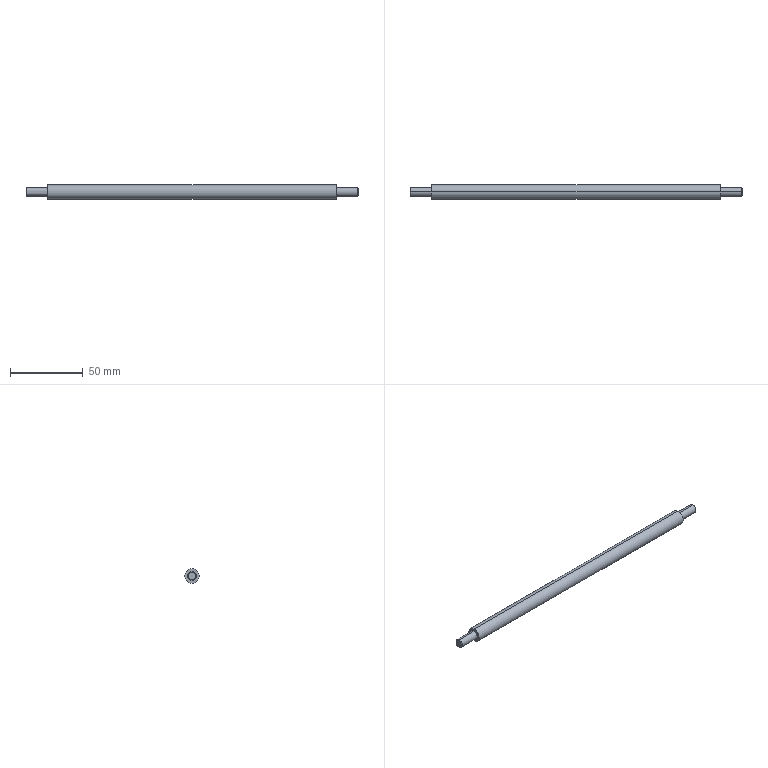Part | STEP file | sliding shaft_SUS304 | 1 solid | 14 faces | box 228 x 10 x 10 mm | volume 16395 mm3 | cylinder 6 | cone 4 | plane 4 | commonest cylinder face diameters 6 x4 10 x2
STEP:
#1=CARTESIAN_POINT('',(0.,0.,0.));
#2=DIRECTION('',(0.,0.,1.));
#3=DIRECTION('',(1.,0.,0.));
#4=AXIS2_PLACEMENT_3D('',#1,#2,#3);
#5=CARTESIAN_POINT('',(198.,0.,5.));
#6=VERTEX_POINT('',#5);
#7=CARTESIAN_POINT('',(198.,0.,-5.));
#8=VERTEX_POINT('',#7);
#9=CARTESIAN_POINT('',(198.,0.,0.));
#10=DIRECTION('',(-1.,0.,0.));
#11=DIRECTION('',(0.,0.,1.));
#12=AXIS2_PLACEMENT_3D('',#9,#10,#11);
#13=CIRCLE('',#12,5.);
#14=CARTESIAN_POINT('',(198.,0.,0.));
#15=DIRECTION('',(-1.,0.,0.));
#16=DIRECTION('',(0.,0.,1.));
#17=AXIS2_PLACEMENT_3D('',#14,#15,#16);
#18=CYLINDRICAL_SURFACE('',#17,5.);
#19=CARTESIAN_POINT('',(0.,0.));
#20=DIRECTION('',(1.,0.));
#21=VECTOR('',#20,1.);
#22=LINE('',#19,#21);
#23=(GEOMETRIC_REPRESENTATION_CONTEXT(2)PARAMETRIC_REPRESENTATION_CONTEXT()REPRESENTATION_CONTEXT('',''));
#24=DEFINITIONAL_REPRESENTATION('',(#22),#23);
#25=PCURVE('',#18,#24);
#26=CARTESIAN_POINT('',(198.,0.,0.));
#27=DIRECTION('',(1.,0.,0.));
#28=DIRECTION('',(0.,0.,-1.));
#29=AXIS2_PLACEMENT_3D('',#26,#27,#28);
#30=PLANE('',#29);
#31=CARTESIAN_POINT('',(-5.,0.));
#32=CARTESIAN_POINT('',(-5.,8.66));
#33=CARTESIAN_POINT('',(2.5,4.33));
#34=CARTESIAN_POINT('',(10.,0.));
#35=CARTESIAN_POINT('',(2.5,-4.33));
#36=CARTESIAN_POINT('',(-5.,-8.66));
#37=CARTESIAN_POINT('',(-5.,0.));
#38=(BOUNDED_CURVE()B_SPLINE_CURVE(2,(#31,#32,#33,#34,#35,#36,#37),.UNSPECIFIED.,.T.,.F.)B_SPLINE_CURVE_WITH_KNOTS((1,2,2,2,2,1),(-2.094,0.,2.094,4.189,6.283,8.378),.UNSPECIFIED.)CURVE()GEOMETRIC_REPRESENTATION_ITEM()RATIONAL_B_SPLINE_CURVE((1.,0.5,1.,0.5,1.,0.5,1.))REPRESENTATION_ITEM(''));
#39=(GEOMETRIC_REPRESENTATION_CONTEXT(2)PARAMETRIC_REPRESENTATION_CONTEXT()REPRESENTATION_CONTEXT('',''));
#40=DEFINITIONAL_REPRESENTATION('',(#38),#39);
#41=PCURVE('',#30,#40);
#42=SURFACE_CURVE('',#13,(#25,#41),.PCURVE_S1.);
#43=EDGE_CURVE('',#6,#8,#42,.T.);
#44=ORIENTED_EDGE('',*,*,#43,.T.);
#45=CARTESIAN_POINT('',(0.,0.,-5.));
#46=VERTEX_POINT('',#45);
#47=CARTESIAN_POINT('',(198.,0.,-5.));
#48=DIRECTION('',(-1.,0.,0.));
#49=VECTOR('',#48,1.);
#50=LINE('',#47,#49);
#51=CARTESIAN_POINT('',(3.142,0.));
#52=DIRECTION('',(0.,1.));
#53=VECTOR('',#52,1.);
#54=LINE('',#51,#53);
#55=(GEOMETRIC_REPRESENTATION_CONTEXT(2)PARAMETRIC_REPRESENTATION_CONTEXT()REPRESENTATION_CONTEXT('',''));
#56=DEFINITIONAL_REPRESENTATION('',(#54),#55);
#57=PCURVE('',#18,#56);
#58=CARTESIAN_POINT('',(198.,0.,0.));
#59=DIRECTION('',(-1.,0.,0.));
#60=DIRECTION('',(0.,0.,1.));
#61=AXIS2_PLACEMENT_3D('',#58,#59,#60);
#62=CYLINDRICAL_SURFACE('',#61,5.);
#63=CARTESIAN_POINT('',(3.142,0.));
#64=DIRECTION('',(0.,1.));
#65=VECTOR('',#64,1.);
#66=LINE('',#63,#65);
#67=(GEOMETRIC_REPRESENTATION_CONTEXT(2)PARAMETRIC_REPRESENTATION_CONTEXT()REPRESENTATION_CONTEXT('',''));
#68=DEFINITIONAL_REPRESENTATION('',(#66),#67);
#69=PCURVE('',#62,#68);
#70=SURFACE_CURVE('',#50,(#57,#69),.PCURVE_S1.);
#71=EDGE_CURVE('',#8,#46,#70,.T.);
#72=ORIENTED_EDGE('',*,*,#71,.T.);
#73=CARTESIAN_POINT('',(0.,0.,5.));
#74=VERTEX_POINT('',#73);
#75=CARTESIAN_POINT('',(0.,0.,0.));
#76=DIRECTION('',(1.,0.,0.));
#77=DIRECTION('',(0.,0.,1.));
#78=AXIS2_PLACEMENT_3D('',#75,#76,#77);
#79=CIRCLE('',#78,5.);
#80=CARTESIAN_POINT('',(6.283,198.));
#81=DIRECTION('',(-1.,0.));
#82=VECTOR('',#81,1.);
#83=LINE('',#80,#82);
#84=(GEOMETRIC_REPRESENTATION_CONTEXT(2)PARAMETRIC_REPRESENTATION_CONTEXT()REPRESENTATION_CONTEXT('',''));
#85=DEFINITIONAL_REPRESENTATION('',(#83),#84);
#86=PCURVE('',#18,#85);
#87=CARTESIAN_POINT('',(0.,0.,0.));
#88=DIRECTION('',(1.,0.,0.));
#89=DIRECTION('',(0.,0.,-1.));
#90=AXIS2_PLACEMENT_3D('',#87,#88,#89);
#91=PLANE('',#90);
#92=CARTESIAN_POINT('',(0.,0.));
#93=DIRECTION('',(-1.,0.));
#94=AXIS2_PLACEMENT_2D('',#92,#93);
#95=CIRCLE('',#94,5.);
#96=(GEOMETRIC_REPRESENTATION_CONTEXT(2)PARAMETRIC_REPRESENTATION_CONTEXT()REPRESENTATION_CONTEXT('',''));
#97=DEFINITIONAL_REPRESENTATION('',(#95),#96);
#98=PCURVE('',#91,#97);
#99=SURFACE_CURVE('',#79,(#86,#98),.PCURVE_S1.);
#100=EDGE_CURVE('',#46,#74,#99,.T.);
#101=ORIENTED_EDGE('',*,*,#100,.T.);
#102=CARTESIAN_POINT('',(198.,0.,5.));
#103=DIRECTION('',(-1.,0.,0.));
#104=VECTOR('',#103,1.);
#105=LINE('',#102,#104);
#106=CARTESIAN_POINT('',(0.,0.));
#107=DIRECTION('',(0.,1.));
#108=VECTOR('',#107,1.);
#109=LINE('',#106,#108);
#110=(GEOMETRIC_REPRESENTATION_CONTEXT(2)PARAMETRIC_REPRESENTATION_CONTEXT()REPRESENTATION_CONTEXT('',''));
#111=DEFINITIONAL_REPRESENTATION('',(#109),#110);
#112=PCURVE('',#18,#111);
#113=CARTESIAN_POINT('',(6.283,0.));
#114=DIRECTION('',(0.,1.));
#115=VECTOR('',#114,1.);
#116=LINE('',#113,#115);
#117=(GEOMETRIC_REPRESENTATION_CONTEXT(2)PARAMETRIC_REPRESENTATION_CONTEXT()REPRESENTATION_CONTEXT('',''));
#118=DEFINITIONAL_REPRESENTATION('',(#116),#117);
#119=PCURVE('',#62,#118);
#120=SURFACE_CURVE('',#105,(#112,#119),.PCURVE_S1.);
#121=EDGE_CURVE('',#6,#74,#120,.T.);
#122=ORIENTED_EDGE('',*,*,#121,.F.);
#123=EDGE_LOOP('',(#44,#72,#101,#122));
#124=FACE_BOUND('',#123,.T.);
#125=ADVANCED_FACE('',(#124),#18,.T.);
#126=CARTESIAN_POINT('',(-14.5,0.,-3.));
#127=VERTEX_POINT('',#126);
#128=CARTESIAN_POINT('',(-14.5,0.,3.));
#129=VERTEX_POINT('',#128);
#130=CARTESIAN_POINT('',(-14.5,0.,0.));
#131=DIRECTION('',(1.,0.,0.));
#132=DIRECTION('',(0.,0.,-1.));
#133=AXIS2_PLACEMENT_3D('',#130,#131,#132);
#134=CIRCLE('',#133,3.);
#135=CARTESIAN_POINT('',(-15.,0.,0.));
#136=DIRECTION('',(1.,0.,0.));
#137=DIRECTION('',(0.,0.,-1.));
#138=AXIS2_PLACEMENT_3D('',#135,#136,#137);
#139=CYLINDRICAL_SURFACE('',#138,3.);
#140=CARTESIAN_POINT('',(0.,0.5));
#141=DIRECTION('',(1.,0.));
#142=VECTOR('',#141,1.);
#143=LINE('',#140,#142);
#144=(GEOMETRIC_REPRESENTATION_CONTEXT(2)PARAMETRIC_REPRESENTATION_CONTEXT()REPRESENTATION_CONTEXT('',''));
#145=DEFINITIONAL_REPRESENTATION('',(#143),#144);
#146=PCURVE('',#139,#145);
#147=CARTESIAN_POINT('',(-14.5,0.,0.));
#148=DIRECTION('',(1.,0.,0.));
#149=DIRECTION('',(0.,0.,-1.));
#150=AXIS2_PLACEMENT_3D('',#147,#148,#149);
#151=CONICAL_SURFACE('',#150,3.,0.7854);
#152=CARTESIAN_POINT('',(0.,0.));
#153=DIRECTION('',(1.,0.));
#154=VECTOR('',#153,1.);
#155=LINE('',#152,#154);
#156=(GEOMETRIC_REPRESENTATION_CONTEXT(2)PARAMETRIC_REPRESENTATION_CONTEXT()REPRESENTATION_CONTEXT('',''));
#157=DEFINITIONAL_REPRESENTATION('',(#155),#156);
#158=PCURVE('',#151,#157);
#159=SURFACE_CURVE('',#134,(#146,#158),.PCURVE_S1.);
#160=EDGE_CURVE('',#127,#129,#159,.T.);
#161=ORIENTED_EDGE('',*,*,#160,.T.);
#162=CARTESIAN_POINT('',(0.,0.,3.));
#163=VERTEX_POINT('',#162);
#164=CARTESIAN_POINT('',(-15.,0.,3.));
#165=DIRECTION('',(1.,0.,0.));
#166=VECTOR('',#165,1.);
#167=LINE('',#164,#166);
#168=CARTESIAN_POINT('',(3.142,0.));
#169=DIRECTION('',(0.,1.));
#170=VECTOR('',#169,1.);
#171=LINE('',#168,#170);
#172=(GEOMETRIC_REPRESENTATION_CONTEXT(2)PARAMETRIC_REPRESENTATION_CONTEXT()REPRESENTATION_CONTEXT('',''));
#173=DEFINITIONAL_REPRESENTATION('',(#171),#172);
#174=PCURVE('',#139,#173);
#175=CARTESIAN_POINT('',(-15.,0.,0.));
#176=DIRECTION('',(1.,0.,0.));
#177=DIRECTION('',(0.,0.,-1.));
#178=AXIS2_PLACEMENT_3D('',#175,#176,#177);
#179=CYLINDRICAL_SURFACE('',#178,3.);
#180=CARTESIAN_POINT('',(3.142,0.));
#181=DIRECTION('',(0.,1.));
#182=VECTOR('',#181,1.);
#183=LINE('',#180,#182);
#184=(GEOMETRIC_REPRESENTATION_CONTEXT(2)PARAMETRIC_REPRESENTATION_CONTEXT()REPRESENTATION_CONTEXT('',''));
#185=DEFINITIONAL_REPRESENTATION('',(#183),#184);
#186=PCURVE('',#179,#185);
#187=SURFACE_CURVE('',#167,(#174,#186),.PCURVE_S1.);
#188=EDGE_CURVE('',#129,#163,#187,.T.);
#189=ORIENTED_EDGE('',*,*,#188,.T.);
#190=CARTESIAN_POINT('',(0.,0.,-3.));
#191=VERTEX_POINT('',#190);
#192=CARTESIAN_POINT('',(0.,0.,0.));
#193=DIRECTION('',(-1.,0.,0.));
#194=DIRECTION('',(0.,0.,-1.));
#195=AXIS2_PLACEMENT_3D('',#192,#193,#194);
#196=CIRCLE('',#195,3.);
#197=CARTESIAN_POINT('',(6.283,15.));
#198=DIRECTION('',(-1.,0.));
#199=VECTOR('',#198,1.);
#200=LINE('',#197,#199);
#201=(GEOMETRIC_REPRESENTATION_CONTEXT(2)PARAMETRIC_REPRESENTATION_CONTEXT()REPRESENTATION_CONTEXT('',''));
#202=DEFINITIONAL_REPRESENTATION('',(#200),#201);
#203=PCURVE('',#139,#202);
#204=CARTESIAN_POINT('',(3.,0.));
#205=CARTESIAN_POINT('',(3.,-5.196));
#206=CARTESIAN_POINT('',(-1.5,-2.598));
#207=CARTESIAN_POINT('',(-6.,0.));
#208=CARTESIAN_POINT('',(-1.5,2.598));
#209=CARTESIAN_POINT('',(3.,5.196));
#210=CARTESIAN_POINT('',(3.,0.));
#211=(BOUNDED_CURVE()B_SPLINE_CURVE(2,(#204,#205,#206,#207,#208,#209,#210),.UNSPECIFIED.,.T.,.F.)B_SPLINE_CURVE_WITH_KNOTS((1,2,2,2,2,1),(-2.094,0.,2.094,4.189,6.283,8.378),.UNSPECIFIED.)CURVE()GEOMETRIC_REPRESENTATION_ITEM()RATIONAL_B_SPLINE_CURVE((1.,0.5,1.,0.5,1.,0.5,1.))REPRESENTATION_ITEM(''));
#212=(GEOMETRIC_REPRESENTATION_CONTEXT(2)PARAMETRIC_REPRESENTATION_CONTEXT()REPRESENTATION_CONTEXT('',''));
#213=DEFINITIONAL_REPRESENTATION('',(#211),#212);
#214=PCURVE('',#91,#213);
#215=SURFACE_CURVE('',#196,(#203,#214),.PCURVE_S1.);
#216=EDGE_CURVE('',#163,#191,#215,.T.);
#217=ORIENTED_EDGE('',*,*,#216,.T.);
#218=CARTESIAN_POINT('',(-15.,0.,-3.));
#219=DIRECTION('',(1.,0.,0.));
#220=VECTOR('',#219,1.);
#221=LINE('',#218,#220);
#222=CARTESIAN_POINT('',(0.,0.));
#223=DIRECTION('',(0.,1.));
#224=VECTOR('',#223,1.);
#225=LINE('',#222,#224);
#226=(GEOMETRIC_REPRESENTATION_CONTEXT(2)PARAMETRIC_REPRESENTATION_CONTEXT()REPRESENTATION_CONTEXT('',''));
#227=DEFINITIONAL_REPRESENTATION('',(#225),#226);
#228=PCURVE('',#139,#227);
#229=CARTESIAN_POINT('',(6.283,0.));
#230=DIRECTION('',(0.,1.));
#231=VECTOR('',#230,1.);
#232=LINE('',#229,#231);
#233=(GEOMETRIC_REPRESENTATION_CONTEXT(2)PARAMETRIC_REPRESENTATION_CONTEXT()REPRESENTATION_CONTEXT('',''));
#234=DEFINITIONAL_REPRESENTATION('',(#232),#233);
#235=PCURVE('',#179,#234);
#236=SURFACE_CURVE('',#221,(#228,#235),.PCURVE_S1.);
#237=EDGE_CURVE('',#127,#191,#236,.T.);
#238=ORIENTED_EDGE('',*,*,#237,.F.);
#239=EDGE_LOOP('',(#161,#189,#217,#238));
#240=FACE_BOUND('',#239,.T.);
#241=ADVANCED_FACE('',(#240),#139,.T.);
#242=CARTESIAN_POINT('',(212.5,3.,0.));
#243=VERTEX_POINT('',#242);
#244=CARTESIAN_POINT('',(212.5,0.,-3.));
#245=VERTEX_POINT('',#244);
#246=CARTESIAN_POINT('',(212.5,0.,0.));
#247=DIRECTION('',(-1.,0.,0.));
#248=DIRECTION('',(0.,0.,1.));
#249=AXIS2_PLACEMENT_3D('',#246,#247,#248);
#250=CIRCLE('',#249,3.);
#251=CARTESIAN_POINT('',(213.,0.,0.));
#252=DIRECTION('',(-1.,0.,0.));
#253=DIRECTION('',(0.,0.,1.));
#254=AXIS2_PLACEMENT_3D('',#251,#252,#253);
#255=CYLINDRICAL_SURFACE('',#254,3.);
#256=CARTESIAN_POINT('',(0.,0.5));
#257=DIRECTION('',(1.,0.));
#258=VECTOR('',#257,1.);
#259=LINE('',#256,#258);
#260=(GEOMETRIC_REPRESENTATION_CONTEXT(2)PARAMETRIC_REPRESENTATION_CONTEXT()REPRESENTATION_CONTEXT('',''));
#261=DEFINITIONAL_REPRESENTATION('',(#259),#260);
#262=PCURVE('',#255,#261);
#263=CARTESIAN_POINT('',(212.5,0.,0.));
#264=DIRECTION('',(-1.,0.,0.));
#265=DIRECTION('',(0.,-1.,0.));
#266=AXIS2_PLACEMENT_3D('',#263,#264,#265);
#267=CONICAL_SURFACE('',#266,3.,0.7854);
#268=CARTESIAN_POINT('',(1.571,0.));
#269=DIRECTION('',(1.,0.));
#270=VECTOR('',#269,1.);
#271=LINE('',#268,#270);
#272=(GEOMETRIC_REPRESENTATION_CONTEXT(2)PARAMETRIC_REPRESENTATION_CONTEXT()REPRESENTATION_CONTEXT('',''));
#273=DEFINITIONAL_REPRESENTATION('',(#271),#272);
#274=PCURVE('',#267,#273);
#275=SURFACE_CURVE('',#250,(#262,#274),.PCURVE_S1.);
#276=EDGE_CURVE('',#243,#245,#275,.T.);
#277=ORIENTED_EDGE('',*,*,#276,.T.);
#278=CARTESIAN_POINT('',(198.,0.,-3.));
#279=VERTEX_POINT('',#278);
#280=CARTESIAN_POINT('',(213.,0.,-3.));
#281=DIRECTION('',(-1.,0.,0.));
#282=VECTOR('',#281,1.);
#283=LINE('',#280,#282);
#284=CARTESIAN_POINT('',(3.142,0.));
#285=DIRECTION('',(0.,1.));
#286=VECTOR('',#285,1.);
#287=LINE('',#284,#286);
#288=(GEOMETRIC_REPRESENTATION_CONTEXT(2)PARAMETRIC_REPRESENTATION_CONTEXT()REPRESENTATION_CONTEXT('',''));
#289=DEFINITIONAL_REPRESENTATION('',(#287),#288);
#290=PCURVE('',#255,#289);
#291=CARTESIAN_POINT('',(213.,0.,0.));
#292=DIRECTION('',(-1.,0.,0.));
#293=DIRECTION('',(0.,0.,1.));
#294=AXIS2_PLACEMENT_3D('',#291,#292,#293);
#295=CYLINDRICAL_SURFACE('',#294,3.);
#296=CARTESIAN_POINT('',(3.142,0.));
#297=DIRECTION('',(0.,1.));
#298=VECTOR('',#297,1.);
#299=LINE('',#296,#298);
#300=(GEOMETRIC_REPRESENTATION_CONTEXT(2)PARAMETRIC_REPRESENTATION_CONTEXT()REPRESENTATION_CONTEXT('',''));
#301=DEFINITIONAL_REPRESENTATION('',(#299),#300);
#302=PCURVE('',#295,#301);
#303=SURFACE_CURVE('',#283,(#290,#302),.PCURVE_S1.);
#304=EDGE_CURVE('',#245,#279,#303,.T.);
#305=ORIENTED_EDGE('',*,*,#304,.T.);
#306=CARTESIAN_POINT('',(198.,0.,3.));
#307=VERTEX_POINT('',#306);
#308=CARTESIAN_POINT('',(198.,0.,0.));
#309=DIRECTION('',(-1.,0.,0.));
#310=DIRECTION('',(0.,0.,1.));
#311=AXIS2_PLACEMENT_3D('',#308,#309,#310);
#312=CIRCLE('',#311,3.);
#313=CARTESIAN_POINT('',(0.,15.));
#314=DIRECTION('',(1.,0.));
#315=VECTOR('',#314,1.);
#316=LINE('',#313,#315);
#317=(GEOMETRIC_REPRESENTATION_CONTEXT(2)PARAMETRIC_REPRESENTATION_CONTEXT()REPRESENTATION_CONTEXT('',''));
#318=DEFINITIONAL_REPRESENTATION('',(#316),#317);
#319=PCURVE('',#255,#318);
#320=CARTESIAN_POINT('',(-3.,0.));
#321=CARTESIAN_POINT('',(-3.,5.196));
#322=CARTESIAN_POINT('',(1.5,2.598));
#323=CARTESIAN_POINT('',(6.,0.));
#324=CARTESIAN_POINT('',(1.5,-2.598));
#325=CARTESIAN_POINT('',(-3.,-5.196));
#326=CARTESIAN_POINT('',(-3.,0.));
#327=(BOUNDED_CURVE()B_SPLINE_CURVE(2,(#320,#321,#322,#323,#324,#325,#326),.UNSPECIFIED.,.T.,.F.)B_SPLINE_CURVE_WITH_KNOTS((1,2,2,2,2,1),(-2.094,0.,2.094,4.189,6.283,8.378),.UNSPECIFIED.)CURVE()GEOMETRIC_REPRESENTATION_ITEM()RATIONAL_B_SPLINE_CURVE((1.,0.5,1.,0.5,1.,0.5,1.))REPRESENTATION_ITEM(''));
#328=(GEOMETRIC_REPRESENTATION_CONTEXT(2)PARAMETRIC_REPRESENTATION_CONTEXT()REPRESENTATION_CONTEXT('',''));
#329=DEFINITIONAL_REPRESENTATION('',(#327),#328);
#330=PCURVE('',#30,#329);
#331=SURFACE_CURVE('',#312,(#319,#330),.PCURVE_S1.);
#332=EDGE_CURVE('',#307,#279,#331,.T.);
#333=ORIENTED_EDGE('',*,*,#332,.F.);
#334=CARTESIAN_POINT('',(212.5,0.,3.));
#335=VERTEX_POINT('',#334);
#336=CARTESIAN_POINT('',(213.,0.,3.));
#337=DIRECTION('',(-1.,0.,0.));
#338=VECTOR('',#337,1.);
#339=LINE('',#336,#338);
#340=CARTESIAN_POINT('',(0.,0.));
#341=DIRECTION('',(0.,1.));
#342=VECTOR('',#341,1.);
#343=LINE('',#340,#342);
#344=(GEOMETRIC_REPRESENTATION_CONTEXT(2)PARAMETRIC_REPRESENTATION_CONTEXT()REPRESENTATION_CONTEXT('',''));
#345=DEFINITIONAL_REPRESENTATION('',(#343),#344);
#346=PCURVE('',#255,#345);
#347=CARTESIAN_POINT('',(6.283,0.));
#348=DIRECTION('',(0.,1.));
#349=VECTOR('',#348,1.);
#350=LINE('',#347,#349);
#351=(GEOMETRIC_REPRESENTATION_CONTEXT(2)PARAMETRIC_REPRESENTATION_CONTEXT()REPRESENTATION_CONTEXT('',''));
#352=DEFINITIONAL_REPRESENTATION('',(#350),#351);
#353=PCURVE('',#295,#352);
#354=SURFACE_CURVE('',#339,(#346,#353),.PCURVE_S1.);
#355=EDGE_CURVE('',#335,#307,#354,.T.);
#356=ORIENTED_EDGE('',*,*,#355,.F.);
#357=CARTESIAN_POINT('',(212.5,0.,0.));
#358=DIRECTION('',(-1.,0.,0.));
#359=DIRECTION('',(0.,0.,1.));
#360=AXIS2_PLACEMENT_3D('',#357,#358,#359);
#361=CIRCLE('',#360,3.);
#362=CARTESIAN_POINT('',(0.,0.5));
#363=DIRECTION('',(1.,0.));
#364=VECTOR('',#363,1.);
#365=LINE('',#362,#364);
#366=(GEOMETRIC_REPRESENTATION_CONTEXT(2)PARAMETRIC_REPRESENTATION_CONTEXT()REPRESENTATION_CONTEXT('',''));
#367=DEFINITIONAL_REPRESENTATION('',(#365),#366);
#368=PCURVE('',#255,#367);
#369=CARTESIAN_POINT('',(212.5,0.,0.));
#370=DIRECTION('',(-1.,0.,0.));
#371=DIRECTION('',(0.,-1.,0.));
#372=AXIS2_PLACEMENT_3D('',#369,#370,#371);
#373=CONICAL_SURFACE('',#372,3.,0.7854);
#374=CARTESIAN_POINT('',(1.571,0.));
#375=DIRECTION('',(1.,0.));
#376=VECTOR('',#375,1.);
#377=LINE('',#374,#376);
#378=(GEOMETRIC_REPRESENTATION_CONTEXT(2)PARAMETRIC_REPRESENTATION_CONTEXT()REPRESENTATION_CONTEXT('',''));
#379=DEFINITIONAL_REPRESENTATION('',(#377),#378);
#380=PCURVE('',#373,#379);
#381=SURFACE_CURVE('',#361,(#368,#380),.PCURVE_S1.);
#382=EDGE_CURVE('',#335,#243,#381,.T.);
#383=ORIENTED_EDGE('',*,*,#382,.T.);
#384=EDGE_LOOP('',(#277,#305,#333,#356,#383));
#385=FACE_BOUND('',#384,.T.);
#386=ADVANCED_FACE('',(#385),#255,.T.);
#387=CARTESIAN_POINT('',(-15.,0.,-2.5));
#388=VERTEX_POINT('',#387);
#389=CARTESIAN_POINT('',(-15.,0.,2.5));
#390=VERTEX_POINT('',#389);
#391=CARTESIAN_POINT('',(-15.,0.,0.));
#392=DIRECTION('',(1.,0.,0.));
#393=DIRECTION('',(0.,0.,-1.));
#394=AXIS2_PLACEMENT_3D('',#391,#392,#393);
#395=CIRCLE('',#394,2.5);
#396=CARTESIAN_POINT('',(0.,-0.5));
#397=DIRECTION('',(1.,0.));
#398=VECTOR('',#397,1.);
#399=LINE('',#396,#398);
#400=(GEOMETRIC_REPRESENTATION_CONTEXT(2)PARAMETRIC_REPRESENTATION_CONTEXT()REPRESENTATION_CONTEXT('',''));
#401=DEFINITIONAL_REPRESENTATION('',(#399),#400);
#402=PCURVE('',#151,#401);
#403=CARTESIAN_POINT('',(-15.,0.,0.));
#404=DIRECTION('',(-1.,0.,0.));
#405=DIRECTION('',(0.,0.,1.));
#406=AXIS2_PLACEMENT_3D('',#403,#404,#405);
#407=PLANE('',#406);
#408=CARTESIAN_POINT('',(-2.5,0.));
#409=CARTESIAN_POINT('',(-2.5,4.33));
#410=CARTESIAN_POINT('',(1.25,2.165));
#411=CARTESIAN_POINT('',(5.,0.));
#412=CARTESIAN_POINT('',(1.25,-2.165));
#413=CARTESIAN_POINT('',(-2.5,-4.33));
#414=CARTESIAN_POINT('',(-2.5,0.));
#415=(BOUNDED_CURVE()B_SPLINE_CURVE(2,(#408,#409,#410,#411,#412,#413,#414),.UNSPECIFIED.,.T.,.F.)B_SPLINE_CURVE_WITH_KNOTS((1,2,2,2,2,1),(-2.094,0.,2.094,4.189,6.283,8.378),.UNSPECIFIED.)CURVE()GEOMETRIC_REPRESENTATION_ITEM()RATIONAL_B_SPLINE_CURVE((1.,0.5,1.,0.5,1.,0.5,1.))REPRESENTATION_ITEM(''));
#416=(GEOMETRIC_REPRESENTATION_CONTEXT(2)PARAMETRIC_REPRESENTATION_CONTEXT()REPRESENTATION_CONTEXT('',''));
#417=DEFINITIONAL_REPRESENTATION('',(#415),#416);
#418=PCURVE('',#407,#417);
#419=SURFACE_CURVE('',#395,(#402,#418),.PCURVE_S1.);
#420=EDGE_CURVE('',#388,#390,#419,.T.);
#421=ORIENTED_EDGE('',*,*,#420,.T.);
#422=CARTESIAN_POINT('',(-14.5,0.,3.));
#423=DIRECTION('',(0.7071,0.,0.7071));
#424=VECTOR('',#423,1.);
#425=LINE('',#422,#424);
#426=CARTESIAN_POINT('',(3.142,0.));
#427=DIRECTION('',(0.,1.));
#428=VECTOR('',#427,1.);
#429=LINE('',#426,#428);
#430=(GEOMETRIC_REPRESENTATION_CONTEXT(2)PARAMETRIC_REPRESENTATION_CONTEXT()REPRESENTATION_CONTEXT('',''));
#431=DEFINITIONAL_REPRESENTATION('',(#429),#430);
#432=PCURVE('',#151,#431);
#433=CARTESIAN_POINT('',(-14.5,0.,0.));
#434=DIRECTION('',(1.,0.,0.));
#435=DIRECTION('',(0.,0.,-1.));
#436=AXIS2_PLACEMENT_3D('',#433,#434,#435);
#437=CONICAL_SURFACE('',#436,3.,0.7854);
#438=CARTESIAN_POINT('',(3.142,0.));
#439=DIRECTION('',(0.,1.));
#440=VECTOR('',#439,1.);
#441=LINE('',#438,#440);
#442=(GEOMETRIC_REPRESENTATION_CONTEXT(2)PARAMETRIC_REPRESENTATION_CONTEXT()REPRESENTATION_CONTEXT('',''));
#443=DEFINITIONAL_REPRESENTATION('',(#441),#442);
#444=PCURVE('',#437,#443);
#445=SURFACE_CURVE('',#425,(#432,#444),.PCURVE_S1.);
#446=EDGE_CURVE('',#390,#129,#445,.T.);
#447=ORIENTED_EDGE('',*,*,#446,.T.);
#448=ORIENTED_EDGE('',*,*,#160,.F.);
#449=CARTESIAN_POINT('',(-14.5,0.,-3.));
#450=DIRECTION('',(0.7071,0.,-0.7071));
#451=VECTOR('',#450,1.);
#452=LINE('',#449,#451);
#453=CARTESIAN_POINT('',(0.,0.));
#454=DIRECTION('',(0.,1.));
#455=VECTOR('',#454,1.);
#456=LINE('',#453,#455);
#457=(GEOMETRIC_REPRESENTATION_CONTEXT(2)PARAMETRIC_REPRESENTATION_CONTEXT()REPRESENTATION_CONTEXT('',''));
#458=DEFINITIONAL_REPRESENTATION('',(#456),#457);
#459=PCURVE('',#151,#458);
#460=CARTESIAN_POINT('',(6.283,0.));
#461=DIRECTION('',(0.,1.));
#462=VECTOR('',#461,1.);
#463=LINE('',#460,#462);
#464=(GEOMETRIC_REPRESENTATION_CONTEXT(2)PARAMETRIC_REPRESENTATION_CONTEXT()REPRESENTATION_CONTEXT('',''));
#465=DEFINITIONAL_REPRESENTATION('',(#463),#464);
#466=PCURVE('',#437,#465);
#467=SURFACE_CURVE('',#452,(#459,#466),.PCURVE_S1.);
#468=EDGE_CURVE('',#388,#127,#467,.T.);
#469=ORIENTED_EDGE('',*,*,#468,.F.);
#470=EDGE_LOOP('',(#421,#447,#448,#469));
#471=FACE_BOUND('',#470,.T.);
#472=ADVANCED_FACE('',(#471),#151,.T.);
#473=CARTESIAN_POINT('',(213.,-2.5,0.));
#474=VERTEX_POINT('',#473);
#475=CARTESIAN_POINT('',(213.,2.5,0.));
#476=VERTEX_POINT('',#475);
#477=CARTESIAN_POINT('',(213.,0.,0.));
#478=DIRECTION('',(-1.,0.,0.));
#479=DIRECTION('',(0.,-1.,0.));
#480=AXIS2_PLACEMENT_3D('',#477,#478,#479);
#481=CIRCLE('',#480,2.5);
#482=CARTESIAN_POINT('',(0.,-0.5));
#483=DIRECTION('',(1.,0.));
#484=VECTOR('',#483,1.);
#485=LINE('',#482,#484);
#486=(GEOMETRIC_REPRESENTATION_CONTEXT(2)PARAMETRIC_REPRESENTATION_CONTEXT()REPRESENTATION_CONTEXT('',''));
#487=DEFINITIONAL_REPRESENTATION('',(#485),#486);
#488=PCURVE('',#373,#487);
#489=CARTESIAN_POINT('',(213.,0.,0.));
#490=DIRECTION('',(1.,0.,0.));
#491=DIRECTION('',(0.,0.,-1.));
#492=AXIS2_PLACEMENT_3D('',#489,#490,#491);
#493=PLANE('',#492);
#494=CARTESIAN_POINT('',(0.,-2.5));
#495=CARTESIAN_POINT('',(-4.33,-2.5));
#496=CARTESIAN_POINT('',(-2.165,1.25));
#497=CARTESIAN_POINT('',(0.,5.));
#498=CARTESIAN_POINT('',(2.165,1.25));
#499=CARTESIAN_POINT('',(4.33,-2.5));
#500=CARTESIAN_POINT('',(0.,-2.5));
#501=(BOUNDED_CURVE()B_SPLINE_CURVE(2,(#494,#495,#496,#497,#498,#499,#500),.UNSPECIFIED.,.T.,.F.)B_SPLINE_CURVE_WITH_KNOTS((1,2,2,2,2,1),(-2.094,0.,2.094,4.189,6.283,8.378),.UNSPECIFIED.)CURVE()GEOMETRIC_REPRESENTATION_ITEM()RATIONAL_B_SPLINE_CURVE((1.,0.5,1.,0.5,1.,0.5,1.))REPRESENTATION_ITEM(''));
#502=(GEOMETRIC_REPRESENTATION_CONTEXT(2)PARAMETRIC_REPRESENTATION_CONTEXT()REPRESENTATION_CONTEXT('',''));
#503=DEFINITIONAL_REPRESENTATION('',(#501),#502);
#504=PCURVE('',#493,#503);
#505=SURFACE_CURVE('',#481,(#488,#504),.PCURVE_S1.);
#506=EDGE_CURVE('',#474,#476,#505,.T.);
#507=ORIENTED_EDGE('',*,*,#506,.T.);
#508=CARTESIAN_POINT('',(212.5,3.,0.));
#509=DIRECTION('',(-0.7071,0.7071,0.));
#510=VECTOR('',#509,1.);
#511=LINE('',#508,#510);
#512=CARTESIAN_POINT('',(3.142,0.));
#513=DIRECTION('',(0.,1.));
#514=VECTOR('',#513,1.);
#515=LINE('',#512,#514);
#516=(GEOMETRIC_REPRESENTATION_CONTEXT(2)PARAMETRIC_REPRESENTATION_CONTEXT()REPRESENTATION_CONTEXT('',''));
#517=DEFINITIONAL_REPRESENTATION('',(#515),#516);
#518=PCURVE('',#373,#517);
#519=CARTESIAN_POINT('',(3.142,0.));
#520=DIRECTION('',(0.,1.));
#521=VECTOR('',#520,1.);
#522=LINE('',#519,#521);
#523=(GEOMETRIC_REPRESENTATION_CONTEXT(2)PARAMETRIC_REPRESENTATION_CONTEXT()REPRESENTATION_CONTEXT('',''));
#524=DEFINITIONAL_REPRESENTATION('',(#522),#523);
#525=PCURVE('',#267,#524);
#526=SURFACE_CURVE('',#511,(#518,#525),.PCURVE_S1.);
#527=EDGE_CURVE('',#476,#243,#526,.T.);
#528=ORIENTED_EDGE('',*,*,#527,.T.);
#529=ORIENTED_EDGE('',*,*,#382,.F.);
#530=CARTESIAN_POINT('',(212.5,-3.,0.));
#531=VERTEX_POINT('',#530);
#532=CARTESIAN_POINT('',(212.5,0.,0.));
#533=DIRECTION('',(-1.,0.,0.));
#534=DIRECTION('',(0.,0.,1.));
#535=AXIS2_PLACEMENT_3D('',#532,#533,#534);
#536=CIRCLE('',#535,3.);
#537=CARTESIAN_POINT('',(-4.712,0.));
#538=DIRECTION('',(1.,0.));
#539=VECTOR('',#538,1.);
#540=LINE('',#537,#539);
#541=(GEOMETRIC_REPRESENTATION_CONTEXT(2)PARAMETRIC_REPRESENTATION_CONTEXT()REPRESENTATION_CONTEXT('',''));
#542=DEFINITIONAL_REPRESENTATION('',(#540),#541);
#543=PCURVE('',#373,#542);
#544=CARTESIAN_POINT('',(0.,0.5));
#545=DIRECTION('',(1.,0.));
#546=VECTOR('',#545,1.);
#547=LINE('',#544,#546);
#548=(GEOMETRIC_REPRESENTATION_CONTEXT(2)PARAMETRIC_REPRESENTATION_CONTEXT()REPRESENTATION_CONTEXT('',''));
#549=DEFINITIONAL_REPRESENTATION('',(#547),#548);
#550=PCURVE('',#295,#549);
#551=SURFACE_CURVE('',#536,(#543,#550),.PCURVE_S1.);
#552=EDGE_CURVE('',#531,#335,#551,.T.);
#553=ORIENTED_EDGE('',*,*,#552,.F.);
#554=CARTESIAN_POINT('',(212.5,-3.,0.));
#555=DIRECTION('',(-0.7071,-0.7071,0.));
#556=VECTOR('',#555,1.);
#557=LINE('',#554,#556);
#558=CARTESIAN_POINT('',(0.,0.));
#559=DIRECTION('',(0.,1.));
#560=VECTOR('',#559,1.);
#561=LINE('',#558,#560);
#562=(GEOMETRIC_REPRESENTATION_CONTEXT(2)PARAMETRIC_REPRESENTATION_CONTEXT()REPRESENTATION_CONTEXT('',''));
#563=DEFINITIONAL_REPRESENTATION('',(#561),#562);
#564=PCURVE('',#373,#563);
#565=CARTESIAN_POINT('',(6.283,0.));
#566=DIRECTION('',(0.,1.));
#567=VECTOR('',#566,1.);
#568=LINE('',#565,#567);
#569=(GEOMETRIC_REPRESENTATION_CONTEXT(2)PARAMETRIC_REPRESENTATION_CONTEXT()REPRESENTATION_CONTEXT('',''));
#570=DEFINITIONAL_REPRESENTATION('',(#568),#569);
#571=PCURVE('',#267,#570);
#572=SURFACE_CURVE('',#557,(#564,#571),.PCURVE_S1.);
#573=EDGE_CURVE('',#474,#531,#572,.T.);
#574=ORIENTED_EDGE('',*,*,#573,.F.);
#575=EDGE_LOOP('',(#507,#528,#529,#553,#574));
#576=FACE_BOUND('',#575,.T.);
#577=ADVANCED_FACE('',(#576),#373,.T.);
#578=ORIENTED_EDGE('',*,*,#71,.F.);
#579=CARTESIAN_POINT('',(198.,0.,0.));
#580=DIRECTION('',(-1.,0.,0.));
#581=DIRECTION('',(0.,0.,1.));
#582=AXIS2_PLACEMENT_3D('',#579,#580,#581);
#583=CIRCLE('',#582,5.);
#584=CARTESIAN_POINT('',(0.,0.));
#585=DIRECTION('',(1.,0.));
#586=VECTOR('',#585,1.);
#587=LINE('',#584,#586);
#588=(GEOMETRIC_REPRESENTATION_CONTEXT(2)PARAMETRIC_REPRESENTATION_CONTEXT()REPRESENTATION_CONTEXT('',''));
#589=DEFINITIONAL_REPRESENTATION('',(#587),#588);
#590=PCURVE('',#62,#589);
#591=CARTESIAN_POINT('',(-5.,0.));
#592=CARTESIAN_POINT('',(-5.,8.66));
#593=CARTESIAN_POINT('',(2.5,4.33));
#594=CARTESIAN_POINT('',(10.,0.));
#595=CARTESIAN_POINT('',(2.5,-4.33));
#596=CARTESIAN_POINT('',(-5.,-8.66));
#597=CARTESIAN_POINT('',(-5.,0.));
#598=(BOUNDED_CURVE()B_SPLINE_CURVE(2,(#591,#592,#593,#594,#595,#596,#597),.UNSPECIFIED.,.T.,.F.)B_SPLINE_CURVE_WITH_KNOTS((1,2,2,2,2,1),(-2.094,0.,2.094,4.189,6.283,8.378),.UNSPECIFIED.)CURVE()GEOMETRIC_REPRESENTATION_ITEM()RATIONAL_B_SPLINE_CURVE((1.,0.5,1.,0.5,1.,0.5,1.))REPRESENTATION_ITEM(''));
#599=(GEOMETRIC_REPRESENTATION_CONTEXT(2)PARAMETRIC_REPRESENTATION_CONTEXT()REPRESENTATION_CONTEXT('',''));
#600=DEFINITIONAL_REPRESENTATION('',(#598),#599);
#601=PCURVE('',#30,#600);
#602=SURFACE_CURVE('',#583,(#590,#601),.PCURVE_S1.);
#603=EDGE_CURVE('',#8,#6,#602,.T.);
#604=ORIENTED_EDGE('',*,*,#603,.T.);
#605=ORIENTED_EDGE('',*,*,#121,.T.);
#606=CARTESIAN_POINT('',(0.,0.,0.));
#607=DIRECTION('',(1.,0.,0.));
#608=DIRECTION('',(0.,0.,1.));
#609=AXIS2_PLACEMENT_3D('',#606,#607,#608);
#610=CIRCLE('',#609,5.);
#611=CARTESIAN_POINT('',(6.283,198.));
#612=DIRECTION('',(-1.,0.));
#613=VECTOR('',#612,1.);
#614=LINE('',#611,#613);
#615=(GEOMETRIC_REPRESENTATION_CONTEXT(2)PARAMETRIC_REPRESENTATION_CONTEXT()REPRESENTATION_CONTEXT('',''));
#616=DEFINITIONAL_REPRESENTATION('',(#614),#615);
#617=PCURVE('',#62,#616);
#618=CARTESIAN_POINT('',(0.,0.));
#619=DIRECTION('',(-1.,0.));
#620=AXIS2_PLACEMENT_2D('',#618,#619);
#621=CIRCLE('',#620,5.);
#622=(GEOMETRIC_REPRESENTATION_CONTEXT(2)PARAMETRIC_REPRESENTATION_CONTEXT()REPRESENTATION_CONTEXT('',''));
#623=DEFINITIONAL_REPRESENTATION('',(#621),#622);
#624=PCURVE('',#91,#623);
#625=SURFACE_CURVE('',#610,(#617,#624),.PCURVE_S1.);
#626=EDGE_CURVE('',#74,#46,#625,.T.);
#627=ORIENTED_EDGE('',*,*,#626,.T.);
#628=EDGE_LOOP('',(#578,#604,#605,#627));
#629=FACE_BOUND('',#628,.T.);
#630=ADVANCED_FACE('',(#629),#62,.T.);
#631=ORIENTED_EDGE('',*,*,#626,.F.);
#632=ORIENTED_EDGE('',*,*,#100,.F.);
#633=EDGE_LOOP('',(#631,#632));
#634=FACE_BOUND('',#633,.T.);
#635=CARTESIAN_POINT('',(0.,0.,0.));
#636=DIRECTION('',(-1.,0.,0.));
#637=DIRECTION('',(0.,0.,-1.));
#638=AXIS2_PLACEMENT_3D('',#635,#636,#637);
#639=CIRCLE('',#638,3.);
#640=CARTESIAN_POINT('',(3.,0.));
#641=CARTESIAN_POINT('',(3.,-5.196));
#642=CARTESIAN_POINT('',(-1.5,-2.598));
#643=CARTESIAN_POINT('',(-6.,0.));
#644=CARTESIAN_POINT('',(-1.5,2.598));
#645=CARTESIAN_POINT('',(3.,5.196));
#646=CARTESIAN_POINT('',(3.,0.));
#647=(BOUNDED_CURVE()B_SPLINE_CURVE(2,(#640,#641,#642,#643,#644,#645,#646),.UNSPECIFIED.,.T.,.F.)B_SPLINE_CURVE_WITH_KNOTS((1,2,2,2,2,1),(-2.094,0.,2.094,4.189,6.283,8.378),.UNSPECIFIED.)CURVE()GEOMETRIC_REPRESENTATION_ITEM()RATIONAL_B_SPLINE_CURVE((1.,0.5,1.,0.5,1.,0.5,1.))REPRESENTATION_ITEM(''));
#648=(GEOMETRIC_REPRESENTATION_CONTEXT(2)PARAMETRIC_REPRESENTATION_CONTEXT()REPRESENTATION_CONTEXT('',''));
#649=DEFINITIONAL_REPRESENTATION('',(#647),#648);
#650=PCURVE('',#91,#649);
#651=CARTESIAN_POINT('',(6.283,15.));
#652=DIRECTION('',(-1.,0.));
#653=VECTOR('',#652,1.);
#654=LINE('',#651,#653);
#655=(GEOMETRIC_REPRESENTATION_CONTEXT(2)PARAMETRIC_REPRESENTATION_CONTEXT()REPRESENTATION_CONTEXT('',''));
#656=DEFINITIONAL_REPRESENTATION('',(#654),#655);
#657=PCURVE('',#179,#656);
#658=SURFACE_CURVE('',#639,(#650,#657),.PCURVE_S1.);
#659=EDGE_CURVE('',#191,#163,#658,.T.);
#660=ORIENTED_EDGE('',*,*,#659,.F.);
#661=ORIENTED_EDGE('',*,*,#216,.F.);
#662=EDGE_LOOP('',(#660,#661));
#663=FACE_BOUND('',#662,.T.);
#664=ADVANCED_FACE('',(#634,#663),#91,.F.);
#665=ORIENTED_EDGE('',*,*,#43,.F.);
#666=ORIENTED_EDGE('',*,*,#603,.F.);
#667=EDGE_LOOP('',(#665,#666));
#668=FACE_BOUND('',#667,.T.);
#669=ORIENTED_EDGE('',*,*,#332,.T.);
#670=CARTESIAN_POINT('',(198.,0.,0.));
#671=DIRECTION('',(-1.,0.,0.));
#672=DIRECTION('',(0.,0.,1.));
#673=AXIS2_PLACEMENT_3D('',#670,#671,#672);
#674=CIRCLE('',#673,3.);
#675=CARTESIAN_POINT('',(-3.,0.));
#676=CARTESIAN_POINT('',(-3.,5.196));
#677=CARTESIAN_POINT('',(1.5,2.598));
#678=CARTESIAN_POINT('',(6.,0.));
#679=CARTESIAN_POINT('',(1.5,-2.598));
#680=CARTESIAN_POINT('',(-3.,-5.196));
#681=CARTESIAN_POINT('',(-3.,0.));
#682=(BOUNDED_CURVE()B_SPLINE_CURVE(2,(#675,#676,#677,#678,#679,#680,#681),.UNSPECIFIED.,.T.,.F.)B_SPLINE_CURVE_WITH_KNOTS((1,2,2,2,2,1),(-2.094,0.,2.094,4.189,6.283,8.378),.UNSPECIFIED.)CURVE()GEOMETRIC_REPRESENTATION_ITEM()RATIONAL_B_SPLINE_CURVE((1.,0.5,1.,0.5,1.,0.5,1.))REPRESENTATION_ITEM(''));
#683=(GEOMETRIC_REPRESENTATION_CONTEXT(2)PARAMETRIC_REPRESENTATION_CONTEXT()REPRESENTATION_CONTEXT('',''));
#684=DEFINITIONAL_REPRESENTATION('',(#682),#683);
#685=PCURVE('',#30,#684);
#686=CARTESIAN_POINT('',(0.,15.));
#687=DIRECTION('',(1.,0.));
#688=VECTOR('',#687,1.);
#689=LINE('',#686,#688);
#690=(GEOMETRIC_REPRESENTATION_CONTEXT(2)PARAMETRIC_REPRESENTATION_CONTEXT()REPRESENTATION_CONTEXT('',''));
#691=DEFINITIONAL_REPRESENTATION('',(#689),#690);
#692=PCURVE('',#295,#691);
#693=SURFACE_CURVE('',#674,(#685,#692),.PCURVE_S1.);
#694=EDGE_CURVE('',#279,#307,#693,.T.);
#695=ORIENTED_EDGE('',*,*,#694,.T.);
#696=EDGE_LOOP('',(#669,#695));
#697=FACE_BOUND('',#696,.T.);
#698=ADVANCED_FACE('',(#668,#697),#30,.T.);
#699=ORIENTED_EDGE('',*,*,#188,.F.);
#700=CARTESIAN_POINT('',(-14.5,0.,0.));
#701=DIRECTION('',(1.,0.,0.));
#702=DIRECTION('',(0.,0.,-1.));
#703=AXIS2_PLACEMENT_3D('',#700,#701,#702);
#704=CIRCLE('',#703,3.);
#705=CARTESIAN_POINT('',(0.,0.5));
#706=DIRECTION('',(1.,0.));
#707=VECTOR('',#706,1.);
#708=LINE('',#705,#707);
#709=(GEOMETRIC_REPRESENTATION_CONTEXT(2)PARAMETRIC_REPRESENTATION_CONTEXT()REPRESENTATION_CONTEXT('',''));
#710=DEFINITIONAL_REPRESENTATION('',(#708),#709);
#711=PCURVE('',#179,#710);
#712=CARTESIAN_POINT('',(0.,0.));
#713=DIRECTION('',(1.,0.));
#714=VECTOR('',#713,1.);
#715=LINE('',#712,#714);
#716=(GEOMETRIC_REPRESENTATION_CONTEXT(2)PARAMETRIC_REPRESENTATION_CONTEXT()REPRESENTATION_CONTEXT('',''));
#717=DEFINITIONAL_REPRESENTATION('',(#715),#716);
#718=PCURVE('',#437,#717);
#719=SURFACE_CURVE('',#704,(#711,#718),.PCURVE_S1.);
#720=EDGE_CURVE('',#129,#127,#719,.T.);
#721=ORIENTED_EDGE('',*,*,#720,.T.);
#722=ORIENTED_EDGE('',*,*,#237,.T.);
#723=ORIENTED_EDGE('',*,*,#659,.T.);
#724=EDGE_LOOP('',(#699,#721,#722,#723));
#725=FACE_BOUND('',#724,.T.);
#726=ADVANCED_FACE('',(#725),#179,.T.);
#727=ORIENTED_EDGE('',*,*,#304,.F.);
#728=CARTESIAN_POINT('',(212.5,0.,0.));
#729=DIRECTION('',(-1.,0.,0.));
#730=DIRECTION('',(0.,0.,1.));
#731=AXIS2_PLACEMENT_3D('',#728,#729,#730);
#732=CIRCLE('',#731,3.);
#733=CARTESIAN_POINT('',(0.,0.5));
#734=DIRECTION('',(1.,0.));
#735=VECTOR('',#734,1.);
#736=LINE('',#733,#735);
#737=(GEOMETRIC_REPRESENTATION_CONTEXT(2)PARAMETRIC_REPRESENTATION_CONTEXT()REPRESENTATION_CONTEXT('',''));
#738=DEFINITIONAL_REPRESENTATION('',(#736),#737);
#739=PCURVE('',#295,#738);
#740=CARTESIAN_POINT('',(1.571,0.));
#741=DIRECTION('',(1.,0.));
#742=VECTOR('',#741,1.);
#743=LINE('',#740,#742);
#744=(GEOMETRIC_REPRESENTATION_CONTEXT(2)PARAMETRIC_REPRESENTATION_CONTEXT()REPRESENTATION_CONTEXT('',''));
#745=DEFINITIONAL_REPRESENTATION('',(#743),#744);
#746=PCURVE('',#267,#745);
#747=SURFACE_CURVE('',#732,(#739,#746),.PCURVE_S1.);
#748=EDGE_CURVE('',#245,#531,#747,.T.);
#749=ORIENTED_EDGE('',*,*,#748,.T.);
#750=ORIENTED_EDGE('',*,*,#552,.T.);
#751=ORIENTED_EDGE('',*,*,#355,.T.);
#752=ORIENTED_EDGE('',*,*,#694,.F.);
#753=EDGE_LOOP('',(#727,#749,#750,#751,#752));
#754=FACE_BOUND('',#753,.T.);
#755=ADVANCED_FACE('',(#754),#295,.T.);
#756=ORIENTED_EDGE('',*,*,#446,.F.);
#757=CARTESIAN_POINT('',(-15.,0.,0.));
#758=DIRECTION('',(1.,0.,0.));
#759=DIRECTION('',(0.,0.,-1.));
#760=AXIS2_PLACEMENT_3D('',#757,#758,#759);
#761=CIRCLE('',#760,2.5);
#762=CARTESIAN_POINT('',(0.,-0.5));
#763=DIRECTION('',(1.,0.));
#764=VECTOR('',#763,1.);
#765=LINE('',#762,#764);
#766=(GEOMETRIC_REPRESENTATION_CONTEXT(2)PARAMETRIC_REPRESENTATION_CONTEXT()REPRESENTATION_CONTEXT('',''));
#767=DEFINITIONAL_REPRESENTATION('',(#765),#766);
#768=PCURVE('',#437,#767);
#769=CARTESIAN_POINT('',(-2.5,0.));
#770=CARTESIAN_POINT('',(-2.5,4.33));
#771=CARTESIAN_POINT('',(1.25,2.165));
#772=CARTESIAN_POINT('',(5.,0.));
#773=CARTESIAN_POINT('',(1.25,-2.165));
#774=CARTESIAN_POINT('',(-2.5,-4.33));
#775=CARTESIAN_POINT('',(-2.5,0.));
#776=(BOUNDED_CURVE()B_SPLINE_CURVE(2,(#769,#770,#771,#772,#773,#774,#775),.UNSPECIFIED.,.T.,.F.)B_SPLINE_CURVE_WITH_KNOTS((1,2,2,2,2,1),(-2.094,0.,2.094,4.189,6.283,8.378),.UNSPECIFIED.)CURVE()GEOMETRIC_REPRESENTATION_ITEM()RATIONAL_B_SPLINE_CURVE((1.,0.5,1.,0.5,1.,0.5,1.))REPRESENTATION_ITEM(''));
#777=(GEOMETRIC_REPRESENTATION_CONTEXT(2)PARAMETRIC_REPRESENTATION_CONTEXT()REPRESENTATION_CONTEXT('',''));
#778=DEFINITIONAL_REPRESENTATION('',(#776),#777);
#779=PCURVE('',#407,#778);
#780=SURFACE_CURVE('',#761,(#768,#779),.PCURVE_S1.);
#781=EDGE_CURVE('',#390,#388,#780,.T.);
#782=ORIENTED_EDGE('',*,*,#781,.T.);
#783=ORIENTED_EDGE('',*,*,#468,.T.);
#784=ORIENTED_EDGE('',*,*,#720,.F.);
#785=EDGE_LOOP('',(#756,#782,#783,#784));
#786=FACE_BOUND('',#785,.T.);
#787=ADVANCED_FACE('',(#786),#437,.T.);
#788=ORIENTED_EDGE('',*,*,#527,.F.);
#789=CARTESIAN_POINT('',(213.,0.,0.));
#790=DIRECTION('',(-1.,0.,0.));
#791=DIRECTION('',(0.,-1.,0.));
#792=AXIS2_PLACEMENT_3D('',#789,#790,#791);
#793=CIRCLE('',#792,2.5);
#794=CARTESIAN_POINT('',(0.,-0.5));
#795=DIRECTION('',(1.,0.));
#796=VECTOR('',#795,1.);
#797=LINE('',#794,#796);
#798=(GEOMETRIC_REPRESENTATION_CONTEXT(2)PARAMETRIC_REPRESENTATION_CONTEXT()REPRESENTATION_CONTEXT('',''));
#799=DEFINITIONAL_REPRESENTATION('',(#797),#798);
#800=PCURVE('',#267,#799);
#801=CARTESIAN_POINT('',(0.,-2.5));
#802=CARTESIAN_POINT('',(-4.33,-2.5));
#803=CARTESIAN_POINT('',(-2.165,1.25));
#804=CARTESIAN_POINT('',(0.,5.));
#805=CARTESIAN_POINT('',(2.165,1.25));
#806=CARTESIAN_POINT('',(4.33,-2.5));
#807=CARTESIAN_POINT('',(0.,-2.5));
#808=(BOUNDED_CURVE()B_SPLINE_CURVE(2,(#801,#802,#803,#804,#805,#806,#807),.UNSPECIFIED.,.T.,.F.)B_SPLINE_CURVE_WITH_KNOTS((1,2,2,2,2,1),(-2.094,0.,2.094,4.189,6.283,8.378),.UNSPECIFIED.)CURVE()GEOMETRIC_REPRESENTATION_ITEM()RATIONAL_B_SPLINE_CURVE((1.,0.5,1.,0.5,1.,0.5,1.))REPRESENTATION_ITEM(''));
#809=(GEOMETRIC_REPRESENTATION_CONTEXT(2)PARAMETRIC_REPRESENTATION_CONTEXT()REPRESENTATION_CONTEXT('',''));
#810=DEFINITIONAL_REPRESENTATION('',(#808),#809);
#811=PCURVE('',#493,#810);
#812=SURFACE_CURVE('',#793,(#800,#811),.PCURVE_S1.);
#813=EDGE_CURVE('',#476,#474,#812,.T.);
#814=ORIENTED_EDGE('',*,*,#813,.T.);
#815=ORIENTED_EDGE('',*,*,#573,.T.);
#816=ORIENTED_EDGE('',*,*,#748,.F.);
#817=ORIENTED_EDGE('',*,*,#276,.F.);
#818=EDGE_LOOP('',(#788,#814,#815,#816,#817));
#819=FACE_BOUND('',#818,.T.);
#820=ADVANCED_FACE('',(#819),#267,.T.);
#821=ORIENTED_EDGE('',*,*,#420,.F.);
#822=ORIENTED_EDGE('',*,*,#781,.F.);
#823=EDGE_LOOP('',(#821,#822));
#824=FACE_BOUND('',#823,.T.);
#825=ADVANCED_FACE('',(#824),#407,.T.);
#826=ORIENTED_EDGE('',*,*,#506,.F.);
#827=ORIENTED_EDGE('',*,*,#813,.F.);
#828=EDGE_LOOP('',(#826,#827));
#829=FACE_BOUND('',#828,.T.);
#830=ADVANCED_FACE('',(#829),#493,.T.);
#831=CLOSED_SHELL('',(#125,#241,#386,#472,#577,#630,#664,#698,#726,#755,#787,#820,#825,#830));
#832=MANIFOLD_SOLID_BREP('',#831);
#833=(LENGTH_UNIT()NAMED_UNIT(*)SI_UNIT(.MILLI.,.METRE.));
#834=UNCERTAINTY_MEASURE_WITH_UNIT(LENGTH_MEASURE(0.0000001),#833,'','');
#835=(NAMED_UNIT(*)PLANE_ANGLE_UNIT()SI_UNIT($,.RADIAN.));
#836=(NAMED_UNIT(*)SI_UNIT($,.STERADIAN.)SOLID_ANGLE_UNIT());
#837=(GEOMETRIC_REPRESENTATION_CONTEXT(3)GLOBAL_UNCERTAINTY_ASSIGNED_CONTEXT((#834))GLOBAL_UNIT_ASSIGNED_CONTEXT((#833,#835,#836))REPRESENTATION_CONTEXT('',''));
#838=ADVANCED_BREP_SHAPE_REPRESENTATION('',(#4,#832),#837);